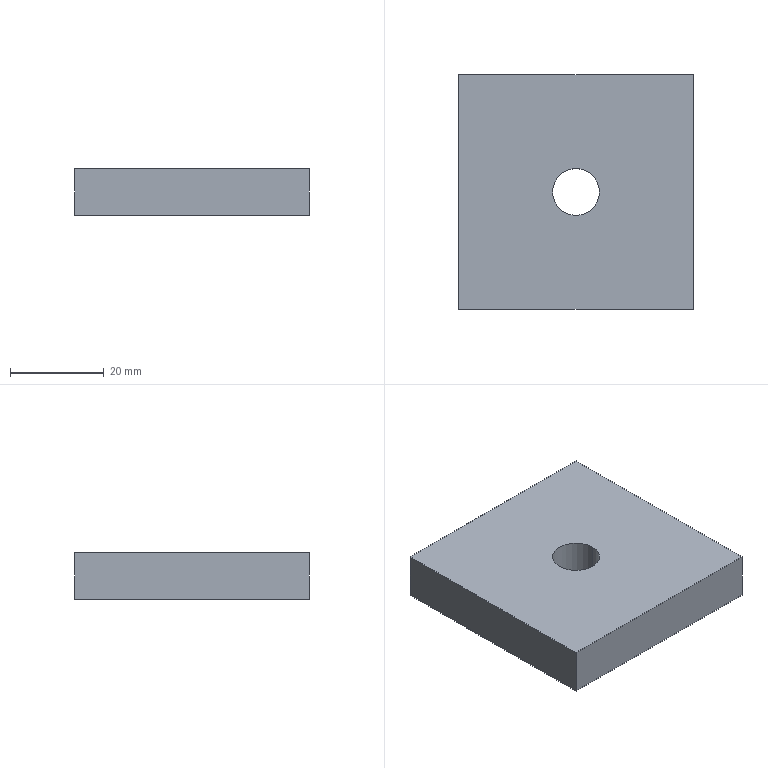Part | SolidWorks | features Extrusion 1 | 1 solid | 8 faces | box 50 x 50 x 10 mm | volume 24215 mm3 | plane 6 | cylinder 2 | commonest cylinder face diameters 10 x2
STEP:
#1=CARTESIAN_POINT('',(20.,25.,10.));
#2=VERTEX_POINT('',#1);
#3=CARTESIAN_POINT('',(30.,25.,10.));
#4=VERTEX_POINT('',#3);
#5=CARTESIAN_POINT('',(25.,25.,10.));
#6=DIRECTION('',(0.,0.,1.));
#7=DIRECTION('',(1.,0.,0.));
#8=AXIS2_PLACEMENT_3D('',#5,#6,#7);
#9=CIRCLE('',#8,5.);
#10=EDGE_CURVE('',#2,#4,#9,.T.);
#11=ORIENTED_EDGE('',*,*,#10,.T.);
#12=CARTESIAN_POINT('',(30.,25.,0.));
#13=VERTEX_POINT('',#12);
#14=CARTESIAN_POINT('',(30.,25.,10.));
#15=DIRECTION('',(0.,0.,-1.));
#16=VECTOR('',#15,1000.);
#17=LINE('',#14,#16);
#18=EDGE_CURVE('',#4,#13,#17,.T.);
#19=ORIENTED_EDGE('',*,*,#18,.T.);
#20=CARTESIAN_POINT('',(20.,25.,0.));
#21=VERTEX_POINT('',#20);
#22=CARTESIAN_POINT('',(25.,25.,0.));
#23=DIRECTION('',(0.,0.,1.));
#24=DIRECTION('',(1.,0.,0.));
#25=AXIS2_PLACEMENT_3D('',#22,#23,#24);
#26=CIRCLE('',#25,5.);
#27=EDGE_CURVE('',#21,#13,#26,.T.);
#28=ORIENTED_EDGE('',*,*,#27,.F.);
#29=CARTESIAN_POINT('',(20.,25.,10.));
#30=DIRECTION('',(0.,0.,-1.));
#31=VECTOR('',#30,1000.);
#32=LINE('',#29,#31);
#33=EDGE_CURVE('',#2,#21,#32,.T.);
#34=ORIENTED_EDGE('',*,*,#33,.F.);
#35=EDGE_LOOP('',(#11,#19,#28,#34));
#36=FACE_OUTER_BOUND('',#35,.T.);
#37=CARTESIAN_POINT('',(25.,25.,10.));
#38=DIRECTION('',(0.,0.,-1.));
#39=DIRECTION('',(-1.,0.,0.));
#40=AXIS2_PLACEMENT_3D('',#37,#38,#39);
#41=CYLINDRICAL_SURFACE('',#40,5.);
#42=ADVANCED_FACE('',(#36),#41,.F.);
#43=CARTESIAN_POINT('',(0.,0.,10.));
#44=VERTEX_POINT('',#43);
#45=CARTESIAN_POINT('',(50.,0.,10.));
#46=VERTEX_POINT('',#45);
#47=CARTESIAN_POINT('',(50.,0.,10.));
#48=DIRECTION('',(1.,0.,0.));
#49=VECTOR('',#48,1000.);
#50=LINE('',#47,#49);
#51=EDGE_CURVE('',#44,#46,#50,.T.);
#52=ORIENTED_EDGE('',*,*,#51,.T.);
#53=CARTESIAN_POINT('',(50.,50.,10.));
#54=VERTEX_POINT('',#53);
#55=CARTESIAN_POINT('',(50.,50.,10.));
#56=DIRECTION('',(0.,1.,0.));
#57=VECTOR('',#56,1000.);
#58=LINE('',#55,#57);
#59=EDGE_CURVE('',#46,#54,#58,.T.);
#60=ORIENTED_EDGE('',*,*,#59,.T.);
#61=CARTESIAN_POINT('',(0.,50.,10.));
#62=VERTEX_POINT('',#61);
#63=CARTESIAN_POINT('',(0.,50.,10.));
#64=DIRECTION('',(-1.,0.,0.));
#65=VECTOR('',#64,1000.);
#66=LINE('',#63,#65);
#67=EDGE_CURVE('',#54,#62,#66,.T.);
#68=ORIENTED_EDGE('',*,*,#67,.T.);
#69=CARTESIAN_POINT('',(0.,0.,10.));
#70=DIRECTION('',(0.,-1.,0.));
#71=VECTOR('',#70,1000.);
#72=LINE('',#69,#71);
#73=EDGE_CURVE('',#62,#44,#72,.T.);
#74=ORIENTED_EDGE('',*,*,#73,.T.);
#75=EDGE_LOOP('',(#52,#60,#68,#74));
#76=FACE_OUTER_BOUND('',#75,.T.);
#77=ORIENTED_EDGE('',*,*,#10,.F.);
#78=CARTESIAN_POINT('',(25.,25.,10.));
#79=DIRECTION('',(0.,0.,1.));
#80=DIRECTION('',(1.,0.,0.));
#81=AXIS2_PLACEMENT_3D('',#78,#79,#80);
#82=CIRCLE('',#81,5.);
#83=EDGE_CURVE('',#4,#2,#82,.T.);
#84=ORIENTED_EDGE('',*,*,#83,.F.);
#85=EDGE_LOOP('',(#77,#84));
#86=FACE_BOUND('',#85,.T.);
#87=CARTESIAN_POINT('',(0.,0.,10.));
#88=DIRECTION('',(0.,0.,-1.));
#89=DIRECTION('',(-1.,0.,0.));
#90=AXIS2_PLACEMENT_3D('',#87,#88,#89);
#91=PLANE('',#90);
#92=ADVANCED_FACE('',(#76,#86),#91,.F.);
#93=CARTESIAN_POINT('',(0.,0.,0.));
#94=VERTEX_POINT('',#93);
#95=CARTESIAN_POINT('',(50.,0.,0.));
#96=VERTEX_POINT('',#95);
#97=CARTESIAN_POINT('',(50.,0.,0.));
#98=DIRECTION('',(1.,0.,0.));
#99=VECTOR('',#98,1000.);
#100=LINE('',#97,#99);
#101=EDGE_CURVE('',#94,#96,#100,.T.);
#102=ORIENTED_EDGE('',*,*,#101,.F.);
#103=CARTESIAN_POINT('',(0.,50.,0.));
#104=VERTEX_POINT('',#103);
#105=CARTESIAN_POINT('',(0.,0.,0.));
#106=DIRECTION('',(0.,-1.,0.));
#107=VECTOR('',#106,1000.);
#108=LINE('',#105,#107);
#109=EDGE_CURVE('',#104,#94,#108,.T.);
#110=ORIENTED_EDGE('',*,*,#109,.F.);
#111=CARTESIAN_POINT('',(50.,50.,0.));
#112=VERTEX_POINT('',#111);
#113=CARTESIAN_POINT('',(0.,50.,0.));
#114=DIRECTION('',(-1.,0.,0.));
#115=VECTOR('',#114,1000.);
#116=LINE('',#113,#115);
#117=EDGE_CURVE('',#112,#104,#116,.T.);
#118=ORIENTED_EDGE('',*,*,#117,.F.);
#119=CARTESIAN_POINT('',(50.,50.,0.));
#120=DIRECTION('',(0.,1.,0.));
#121=VECTOR('',#120,1000.);
#122=LINE('',#119,#121);
#123=EDGE_CURVE('',#96,#112,#122,.T.);
#124=ORIENTED_EDGE('',*,*,#123,.F.);
#125=EDGE_LOOP('',(#102,#110,#118,#124));
#126=FACE_OUTER_BOUND('',#125,.T.);
#127=ORIENTED_EDGE('',*,*,#27,.T.);
#128=CARTESIAN_POINT('',(25.,25.,0.));
#129=DIRECTION('',(0.,0.,1.));
#130=DIRECTION('',(1.,0.,0.));
#131=AXIS2_PLACEMENT_3D('',#128,#129,#130);
#132=CIRCLE('',#131,5.);
#133=EDGE_CURVE('',#13,#21,#132,.T.);
#134=ORIENTED_EDGE('',*,*,#133,.T.);
#135=EDGE_LOOP('',(#127,#134));
#136=FACE_BOUND('',#135,.T.);
#137=CARTESIAN_POINT('',(0.,0.,0.));
#138=DIRECTION('',(0.,0.,-1.));
#139=DIRECTION('',(-1.,0.,0.));
#140=AXIS2_PLACEMENT_3D('',#137,#138,#139);
#141=PLANE('',#140);
#142=ADVANCED_FACE('',(#126,#136),#141,.T.);
#143=ORIENTED_EDGE('',*,*,#101,.T.);
#144=CARTESIAN_POINT('',(50.,0.,10.));
#145=DIRECTION('',(0.,0.,-1.));
#146=VECTOR('',#145,1000.);
#147=LINE('',#144,#146);
#148=EDGE_CURVE('',#46,#96,#147,.T.);
#149=ORIENTED_EDGE('',*,*,#148,.F.);
#150=ORIENTED_EDGE('',*,*,#51,.F.);
#151=CARTESIAN_POINT('',(0.,0.,10.));
#152=DIRECTION('',(0.,0.,-1.));
#153=VECTOR('',#152,1000.);
#154=LINE('',#151,#153);
#155=EDGE_CURVE('',#44,#94,#154,.T.);
#156=ORIENTED_EDGE('',*,*,#155,.T.);
#157=EDGE_LOOP('',(#143,#149,#150,#156));
#158=FACE_OUTER_BOUND('',#157,.T.);
#159=CARTESIAN_POINT('',(50.,0.,10.));
#160=DIRECTION('',(0.,1.,0.));
#161=DIRECTION('',(0.,0.,1.));
#162=AXIS2_PLACEMENT_3D('',#159,#160,#161);
#163=PLANE('',#162);
#164=ADVANCED_FACE('',(#158),#163,.F.);
#165=ORIENTED_EDGE('',*,*,#123,.T.);
#166=CARTESIAN_POINT('',(50.,50.,10.));
#167=DIRECTION('',(0.,0.,-1.));
#168=VECTOR('',#167,1000.);
#169=LINE('',#166,#168);
#170=EDGE_CURVE('',#54,#112,#169,.T.);
#171=ORIENTED_EDGE('',*,*,#170,.F.);
#172=ORIENTED_EDGE('',*,*,#59,.F.);
#173=ORIENTED_EDGE('',*,*,#148,.T.);
#174=EDGE_LOOP('',(#165,#171,#172,#173));
#175=FACE_OUTER_BOUND('',#174,.T.);
#176=CARTESIAN_POINT('',(50.,50.,10.));
#177=DIRECTION('',(-1.,0.,0.));
#178=DIRECTION('',(0.,0.,1.));
#179=AXIS2_PLACEMENT_3D('',#176,#177,#178);
#180=PLANE('',#179);
#181=ADVANCED_FACE('',(#175),#180,.F.);
#182=ORIENTED_EDGE('',*,*,#117,.T.);
#183=CARTESIAN_POINT('',(0.,50.,10.));
#184=DIRECTION('',(0.,0.,-1.));
#185=VECTOR('',#184,1000.);
#186=LINE('',#183,#185);
#187=EDGE_CURVE('',#62,#104,#186,.T.);
#188=ORIENTED_EDGE('',*,*,#187,.F.);
#189=ORIENTED_EDGE('',*,*,#67,.F.);
#190=ORIENTED_EDGE('',*,*,#170,.T.);
#191=EDGE_LOOP('',(#182,#188,#189,#190));
#192=FACE_OUTER_BOUND('',#191,.T.);
#193=CARTESIAN_POINT('',(0.,50.,10.));
#194=DIRECTION('',(0.,-1.,0.));
#195=DIRECTION('',(0.,0.,-1.));
#196=AXIS2_PLACEMENT_3D('',#193,#194,#195);
#197=PLANE('',#196);
#198=ADVANCED_FACE('',(#192),#197,.F.);
#199=ORIENTED_EDGE('',*,*,#109,.T.);
#200=ORIENTED_EDGE('',*,*,#155,.F.);
#201=ORIENTED_EDGE('',*,*,#73,.F.);
#202=ORIENTED_EDGE('',*,*,#187,.T.);
#203=EDGE_LOOP('',(#199,#200,#201,#202));
#204=FACE_OUTER_BOUND('',#203,.T.);
#205=CARTESIAN_POINT('',(0.,0.,10.));
#206=DIRECTION('',(1.,0.,0.));
#207=DIRECTION('',(0.,0.,-1.));
#208=AXIS2_PLACEMENT_3D('',#205,#206,#207);
#209=PLANE('',#208);
#210=ADVANCED_FACE('',(#204),#209,.F.);
#211=ORIENTED_EDGE('',*,*,#18,.F.);
#212=ORIENTED_EDGE('',*,*,#83,.T.);
#213=ORIENTED_EDGE('',*,*,#33,.T.);
#214=ORIENTED_EDGE('',*,*,#133,.F.);
#215=EDGE_LOOP('',(#211,#212,#213,#214));
#216=FACE_OUTER_BOUND('',#215,.T.);
#217=CARTESIAN_POINT('',(25.,25.,10.));
#218=DIRECTION('',(0.,0.,-1.));
#219=DIRECTION('',(-1.,0.,0.));
#220=AXIS2_PLACEMENT_3D('',#217,#218,#219);
#221=CYLINDRICAL_SURFACE('',#220,5.);
#222=ADVANCED_FACE('',(#216),#221,.F.);
#223=CLOSED_SHELL('',(#42,#92,#142,#164,#181,#198,#210,#222));
#224=MANIFOLD_SOLID_BREP('',#223);
#225=CARTESIAN_POINT('',(0.,0.,0.));
#226=DIRECTION('',(0.,0.,1.));
#227=DIRECTION('',(1.,0.,0.));
#228=AXIS2_PLACEMENT_3D('',#225,#226,#227);
#229=(LENGTH_UNIT()NAMED_UNIT(*)SI_UNIT(.MILLI.,.METRE.));
#230=UNCERTAINTY_MEASURE_WITH_UNIT(LENGTH_MEASURE(0.00001),#229,'','');
#231=(NAMED_UNIT(*)PLANE_ANGLE_UNIT()SI_UNIT($,.RADIAN.));
#232=(NAMED_UNIT(*)SI_UNIT($,.STERADIAN.)SOLID_ANGLE_UNIT());
#233=(GEOMETRIC_REPRESENTATION_CONTEXT(3)GLOBAL_UNCERTAINTY_ASSIGNED_CONTEXT((#230))GLOBAL_UNIT_ASSIGNED_CONTEXT((#229,#231,#232))REPRESENTATION_CONTEXT('',''));
#234=ADVANCED_BREP_SHAPE_REPRESENTATION('',(#224,#228),#233);